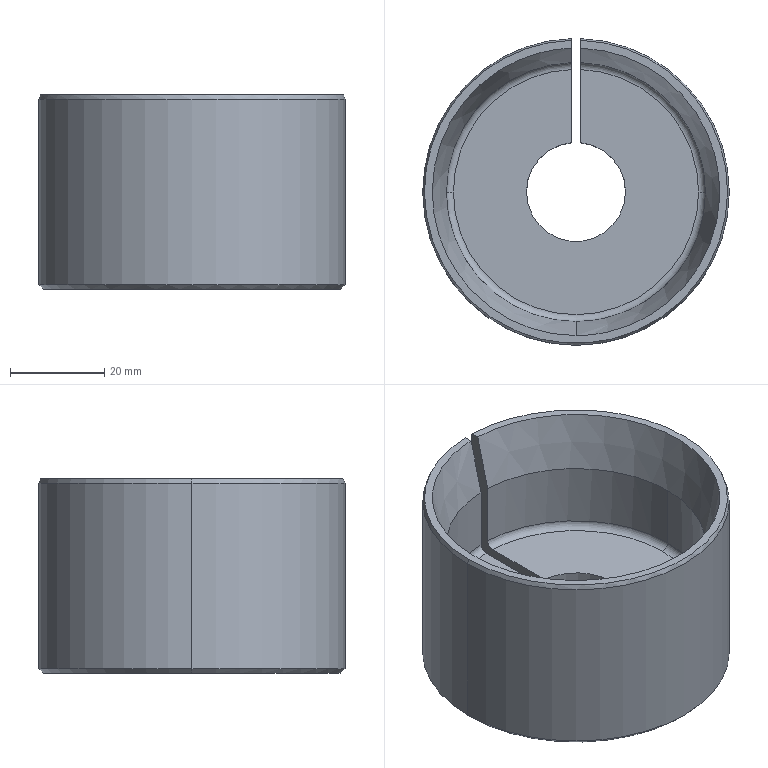Part | SolidWorks | features Chamfer 2, ICE 2, 3DProfileFeature 1, Extrusion 1, Fillet 1, HoleWzd 1, RevCut 1 | 1 solid | 25 faces | box 65 x 64.985 x 41.25 mm | volume 63691 mm3 | cylinder 9 | cone 8 | plane 5 | torus 3 | commonest cylinder face diameters 21 x3 55 x3 65 x3
STEP:
#1=CARTESIAN_POINT('',(-26.,0.,14.25));
#2=VERTEX_POINT('',#1);
#3=CARTESIAN_POINT('',(26.,0.,14.25));
#4=VERTEX_POINT('',#3);
#5=CARTESIAN_POINT('',(0.,0.,14.25));
#6=DIRECTION('',(0.,0.,1.));
#7=DIRECTION('',(1.,0.,0.));
#8=AXIS2_PLACEMENT_3D('',#5,#6,#7);
#9=CIRCLE('',#8,26.);
#10=EDGE_CURVE('',#2,#4,#9,.T.);
#11=ORIENTED_EDGE('',*,*,#10,.F.);
#12=CARTESIAN_POINT('',(-27.5,0.,15.75));
#13=VERTEX_POINT('',#12);
#14=CARTESIAN_POINT('',(-26.,0.,15.75));
#15=DIRECTION('',(0.,1.,0.));
#16=DIRECTION('',(-1.,0.,0.));
#17=AXIS2_PLACEMENT_3D('',#14,#15,#16);
#18=CIRCLE('',#17,1.5);
#19=EDGE_CURVE('',#2,#13,#18,.T.);
#20=ORIENTED_EDGE('',*,*,#19,.T.);
#21=CARTESIAN_POINT('',(27.5,0.,15.75));
#22=VERTEX_POINT('',#21);
#23=CARTESIAN_POINT('',(0.,0.,15.75));
#24=DIRECTION('',(0.,0.,-1.));
#25=DIRECTION('',(1.,0.,0.));
#26=AXIS2_PLACEMENT_3D('',#23,#24,#25);
#27=CIRCLE('',#26,27.5);
#28=EDGE_CURVE('',#22,#13,#27,.T.);
#29=ORIENTED_EDGE('',*,*,#28,.F.);
#30=CARTESIAN_POINT('',(26.,0.,15.75));
#31=DIRECTION('',(0.,-1.,0.));
#32=DIRECTION('',(0.,0.,-1.));
#33=AXIS2_PLACEMENT_3D('',#30,#31,#32);
#34=CIRCLE('',#33,1.5);
#35=EDGE_CURVE('',#4,#22,#34,.T.);
#36=ORIENTED_EDGE('',*,*,#35,.F.);
#37=EDGE_LOOP('',(#11,#20,#29,#36));
#38=FACE_OUTER_BOUND('',#37,.T.);
#39=CARTESIAN_POINT('',(0.,0.,15.75));
#40=DIRECTION('',(0.,0.,1.));
#41=DIRECTION('',(1.,0.,0.));
#42=AXIS2_PLACEMENT_3D('',#39,#40,#41);
#43=TOROIDAL_SURFACE('',#42,26.,1.5);
#44=ADVANCED_FACE('',(#38),#43,.F.);
#45=CARTESIAN_POINT('',(1.,25.981,14.25));
#46=VERTEX_POINT('',#45);
#47=CARTESIAN_POINT('',(0.,0.,14.25));
#48=DIRECTION('',(0.,0.,1.));
#49=DIRECTION('',(1.,0.,0.));
#50=AXIS2_PLACEMENT_3D('',#47,#48,#49);
#51=CIRCLE('',#50,26.);
#52=EDGE_CURVE('',#4,#46,#51,.T.);
#53=ORIENTED_EDGE('',*,*,#52,.F.);
#54=ORIENTED_EDGE('',*,*,#35,.T.);
#55=CARTESIAN_POINT('',(1.,27.482,15.75));
#56=VERTEX_POINT('',#55);
#57=CARTESIAN_POINT('',(0.,0.,15.75));
#58=DIRECTION('',(0.,0.,-1.));
#59=DIRECTION('',(1.,0.,0.));
#60=AXIS2_PLACEMENT_3D('',#57,#58,#59);
#61=CIRCLE('',#60,27.5);
#62=EDGE_CURVE('',#56,#22,#61,.T.);
#63=ORIENTED_EDGE('',*,*,#62,.F.);
#64=CARTESIAN_POINT('',(1.,25.981,14.25));
#65=CARTESIAN_POINT('',(1.,26.08,14.25));
#66=CARTESIAN_POINT('',(1.,26.177,14.26));
#67=CARTESIAN_POINT('',(1.,26.369,14.298));
#68=CARTESIAN_POINT('',(1.,26.464,14.327));
#69=CARTESIAN_POINT('',(1.,26.646,14.402));
#70=CARTESIAN_POINT('',(1.,26.732,14.448));
#71=CARTESIAN_POINT('',(1.,26.895,14.556));
#72=CARTESIAN_POINT('',(1.,26.972,14.62));
#73=CARTESIAN_POINT('',(1.,27.18,14.827));
#74=CARTESIAN_POINT('',(1.,27.292,14.994));
#75=CARTESIAN_POINT('',(1.,27.442,15.355));
#76=CARTESIAN_POINT('',(1.,27.482,15.552));
#77=CARTESIAN_POINT('',(1.,27.482,15.75));
#78=B_SPLINE_CURVE_WITH_KNOTS('',3,(#64,#65,#66,#67,#68,#69,#70,#71,#72,#73,#74,#75,#76,#77),.UNSPECIFIED.,.F.,.F.,(4,2,2,2,2,2,4),(0.,0.000293,0.000586,0.000879,0.001172,0.001758,0.002344),.UNSPECIFIED.);
#79=EDGE_CURVE('',#46,#56,#78,.T.);
#80=ORIENTED_EDGE('',*,*,#79,.F.);
#81=EDGE_LOOP('',(#53,#54,#63,#80));
#82=FACE_OUTER_BOUND('',#81,.T.);
#83=CARTESIAN_POINT('',(0.,0.,15.75));
#84=DIRECTION('',(0.,0.,1.));
#85=DIRECTION('',(1.,0.,0.));
#86=AXIS2_PLACEMENT_3D('',#83,#84,#85);
#87=TOROIDAL_SURFACE('',#86,26.,1.5);
#88=ADVANCED_FACE('',(#82),#87,.F.);
#89=CARTESIAN_POINT('',(32.136,0.,41.25));
#90=VERTEX_POINT('',#89);
#91=CARTESIAN_POINT('',(1.,32.12,41.25));
#92=VERTEX_POINT('',#91);
#93=CARTESIAN_POINT('',(0.,0.,41.25));
#94=DIRECTION('',(0.,0.,1.));
#95=DIRECTION('',(1.,0.,0.));
#96=AXIS2_PLACEMENT_3D('',#93,#94,#95);
#97=CIRCLE('',#96,32.136);
#98=EDGE_CURVE('',#90,#92,#97,.T.);
#99=ORIENTED_EDGE('',*,*,#98,.F.);
#100=CARTESIAN_POINT('',(32.5,0.,40.25));
#101=VERTEX_POINT('',#100);
#102=CARTESIAN_POINT('',(32.136,0.,41.25));
#103=DIRECTION('',(0.342,0.,-0.9397));
#104=VECTOR('',#103,1000.);
#105=LINE('',#102,#104);
#106=EDGE_CURVE('',#90,#101,#105,.T.);
#107=ORIENTED_EDGE('',*,*,#106,.T.);
#108=CARTESIAN_POINT('',(1.,32.485,40.25));
#109=VERTEX_POINT('',#108);
#110=CARTESIAN_POINT('',(0.,0.,40.25));
#111=DIRECTION('',(0.,0.,-1.));
#112=DIRECTION('',(1.,0.,0.));
#113=AXIS2_PLACEMENT_3D('',#110,#111,#112);
#114=CIRCLE('',#113,32.5);
#115=EDGE_CURVE('',#109,#101,#114,.T.);
#116=ORIENTED_EDGE('',*,*,#115,.F.);
#117=CARTESIAN_POINT('',(1.,32.12,41.25));
#118=CARTESIAN_POINT('',(1.,32.242,40.917));
#119=CARTESIAN_POINT('',(1.,32.363,40.583));
#120=CARTESIAN_POINT('',(1.,32.485,40.25));
#121=B_SPLINE_CURVE_WITH_KNOTS('',3,(#117,#118,#119,#120),.UNSPECIFIED.,.F.,.F.,(4,4),(0.,0.001064),.UNSPECIFIED.);
#122=EDGE_CURVE('',#92,#109,#121,.T.);
#123=ORIENTED_EDGE('',*,*,#122,.F.);
#124=EDGE_LOOP('',(#99,#107,#116,#123));
#125=FACE_OUTER_BOUND('',#124,.T.);
#126=CARTESIAN_POINT('',(0.,0.,41.25));
#127=DIRECTION('',(0.,0.,-1.));
#128=DIRECTION('',(-1.,0.,0.));
#129=AXIS2_PLACEMENT_3D('',#126,#127,#128);
#130=CONICAL_SURFACE('',#129,32.136,0.3491);
#131=ADVANCED_FACE('',(#125),#130,.T.);
#132=ORIENTED_EDGE('',*,*,#106,.F.);
#133=CARTESIAN_POINT('',(-32.136,0.,41.25));
#134=VERTEX_POINT('',#133);
#135=CARTESIAN_POINT('',(0.,0.,41.25));
#136=DIRECTION('',(0.,0.,1.));
#137=DIRECTION('',(1.,0.,0.));
#138=AXIS2_PLACEMENT_3D('',#135,#136,#137);
#139=CIRCLE('',#138,32.136);
#140=EDGE_CURVE('',#134,#90,#139,.T.);
#141=ORIENTED_EDGE('',*,*,#140,.F.);
#142=CARTESIAN_POINT('',(-32.5,0.,40.25));
#143=VERTEX_POINT('',#142);
#144=CARTESIAN_POINT('',(-32.136,0.,41.25));
#145=DIRECTION('',(-0.342,0.,-0.9397));
#146=VECTOR('',#145,1000.);
#147=LINE('',#144,#146);
#148=EDGE_CURVE('',#134,#143,#147,.T.);
#149=ORIENTED_EDGE('',*,*,#148,.T.);
#150=CARTESIAN_POINT('',(0.,0.,40.25));
#151=DIRECTION('',(0.,0.,-1.));
#152=DIRECTION('',(1.,0.,0.));
#153=AXIS2_PLACEMENT_3D('',#150,#151,#152);
#154=CIRCLE('',#153,32.5);
#155=EDGE_CURVE('',#101,#143,#154,.T.);
#156=ORIENTED_EDGE('',*,*,#155,.F.);
#157=EDGE_LOOP('',(#132,#141,#149,#156));
#158=FACE_OUTER_BOUND('',#157,.T.);
#159=CARTESIAN_POINT('',(0.,0.,41.25));
#160=DIRECTION('',(0.,0.,-1.));
#161=DIRECTION('',(-1.,0.,0.));
#162=AXIS2_PLACEMENT_3D('',#159,#160,#161);
#163=CONICAL_SURFACE('',#162,32.136,0.3491);
#164=ADVANCED_FACE('',(#158),#163,.T.);
#165=CARTESIAN_POINT('',(-31.5,0.,0.));
#166=VERTEX_POINT('',#165);
#167=CARTESIAN_POINT('',(-1.,31.484,0.));
#168=VERTEX_POINT('',#167);
#169=CARTESIAN_POINT('',(0.,0.,0.));
#170=DIRECTION('',(0.,0.,-1.));
#171=DIRECTION('',(1.,0.,0.));
#172=AXIS2_PLACEMENT_3D('',#169,#170,#171);
#173=CIRCLE('',#172,31.5);
#174=EDGE_CURVE('',#166,#168,#173,.T.);
#175=ORIENTED_EDGE('',*,*,#174,.F.);
#176=CARTESIAN_POINT('',(-32.5,0.,1.));
#177=VERTEX_POINT('',#176);
#178=CARTESIAN_POINT('',(-32.5,0.,1.));
#179=DIRECTION('',(-0.7071,0.,0.7071));
#180=VECTOR('',#179,1000.);
#181=LINE('',#178,#180);
#182=EDGE_CURVE('',#166,#177,#181,.T.);
#183=ORIENTED_EDGE('',*,*,#182,.T.);
#184=CARTESIAN_POINT('',(-1.,32.485,1.));
#185=VERTEX_POINT('',#184);
#186=CARTESIAN_POINT('',(0.,0.,1.));
#187=DIRECTION('',(0.,0.,1.));
#188=DIRECTION('',(1.,0.,0.));
#189=AXIS2_PLACEMENT_3D('',#186,#187,#188);
#190=CIRCLE('',#189,32.5);
#191=EDGE_CURVE('',#185,#177,#190,.T.);
#192=ORIENTED_EDGE('',*,*,#191,.F.);
#193=CARTESIAN_POINT('',(-1.,31.484,0.));
#194=CARTESIAN_POINT('',(-1.,31.818,0.3333));
#195=CARTESIAN_POINT('',(-1.,32.151,0.6667));
#196=CARTESIAN_POINT('',(-1.,32.485,1.));
#197=B_SPLINE_CURVE_WITH_KNOTS('',3,(#193,#194,#195,#196),.UNSPECIFIED.,.F.,.F.,(4,4),(0.,0.001415),.UNSPECIFIED.);
#198=EDGE_CURVE('',#168,#185,#197,.T.);
#199=ORIENTED_EDGE('',*,*,#198,.F.);
#200=EDGE_LOOP('',(#175,#183,#192,#199));
#201=FACE_OUTER_BOUND('',#200,.T.);
#202=CARTESIAN_POINT('',(0.,0.,1.));
#203=DIRECTION('',(0.,0.,1.));
#204=DIRECTION('',(1.,0.,0.));
#205=AXIS2_PLACEMENT_3D('',#202,#203,#204);
#206=CONICAL_SURFACE('',#205,32.5,0.7854);
#207=ADVANCED_FACE('',(#201),#206,.T.);
#208=ORIENTED_EDGE('',*,*,#182,.F.);
#209=CARTESIAN_POINT('',(31.5,0.,0.));
#210=VERTEX_POINT('',#209);
#211=CARTESIAN_POINT('',(0.,0.,0.));
#212=DIRECTION('',(0.,0.,-1.));
#213=DIRECTION('',(1.,0.,0.));
#214=AXIS2_PLACEMENT_3D('',#211,#212,#213);
#215=CIRCLE('',#214,31.5);
#216=EDGE_CURVE('',#210,#166,#215,.T.);
#217=ORIENTED_EDGE('',*,*,#216,.F.);
#218=CARTESIAN_POINT('',(32.5,0.,1.));
#219=VERTEX_POINT('',#218);
#220=CARTESIAN_POINT('',(32.5,0.,1.));
#221=DIRECTION('',(0.7071,0.,0.7071));
#222=VECTOR('',#221,1000.);
#223=LINE('',#220,#222);
#224=EDGE_CURVE('',#210,#219,#223,.T.);
#225=ORIENTED_EDGE('',*,*,#224,.T.);
#226=CARTESIAN_POINT('',(0.,0.,1.));
#227=DIRECTION('',(0.,0.,1.));
#228=DIRECTION('',(1.,0.,0.));
#229=AXIS2_PLACEMENT_3D('',#226,#227,#228);
#230=CIRCLE('',#229,32.5);
#231=EDGE_CURVE('',#177,#219,#230,.T.);
#232=ORIENTED_EDGE('',*,*,#231,.F.);
#233=EDGE_LOOP('',(#208,#217,#225,#232));
#234=FACE_OUTER_BOUND('',#233,.T.);
#235=CARTESIAN_POINT('',(0.,0.,1.));
#236=DIRECTION('',(0.,0.,1.));
#237=DIRECTION('',(1.,0.,0.));
#238=AXIS2_PLACEMENT_3D('',#235,#236,#237);
#239=CONICAL_SURFACE('',#238,32.5,0.7854);
#240=ADVANCED_FACE('',(#234),#239,.T.);
#241=CARTESIAN_POINT('',(27.5,0.,29.296));
#242=VERTEX_POINT('',#241);
#243=CARTESIAN_POINT('',(0.,-27.5,29.269));
#244=VERTEX_POINT('',#243);
#245=CARTESIAN_POINT('',(27.5,0.,29.296));
#246=CARTESIAN_POINT('',(27.5,-0.8956,29.295));
#247=CARTESIAN_POINT('',(27.456,-1.792,29.294));
#248=CARTESIAN_POINT('',(27.28,-3.586,29.292));
#249=CARTESIAN_POINT('',(27.146,-4.488,29.291));
#250=CARTESIAN_POINT('',(26.617,-7.143,29.289));
#251=CARTESIAN_POINT('',(26.096,-8.857,29.287));
#252=CARTESIAN_POINT('',(25.067,-11.346,29.285));
#253=CARTESIAN_POINT('',(24.681,-12.162,29.284));
#254=CARTESIAN_POINT('',(23.825,-13.764,29.282));
#255=CARTESIAN_POINT('',(23.361,-14.537,29.282));
#256=CARTESIAN_POINT('',(21.865,-16.775,29.279));
#257=CARTESIAN_POINT('',(20.729,-18.161,29.278));
#258=CARTESIAN_POINT('',(18.815,-20.077,29.276));
#259=CARTESIAN_POINT('',(18.139,-20.689,29.276));
#260=CARTESIAN_POINT('',(16.746,-21.832,29.274));
#261=CARTESIAN_POINT('',(16.025,-22.366,29.274));
#262=CARTESIAN_POINT('',(14.536,-23.362,29.273));
#263=CARTESIAN_POINT('',(13.768,-23.823,29.273));
#264=CARTESIAN_POINT('',(12.579,-24.458,29.272));
#265=CARTESIAN_POINT('',(12.177,-24.661,29.272));
#266=CARTESIAN_POINT('',(11.36,-25.048,29.271));
#267=CARTESIAN_POINT('',(10.945,-25.232,29.271));
#268=CARTESIAN_POINT('',(8.852,-26.099,29.27));
#269=CARTESIAN_POINT('',(7.135,-26.619,29.27));
#270=CARTESIAN_POINT('',(4.498,-27.144,29.269));
#271=CARTESIAN_POINT('',(3.609,-27.277,29.269));
#272=CARTESIAN_POINT('',(2.259,-27.411,29.269));
#273=CARTESIAN_POINT('',(1.805,-27.444,29.269));
#274=CARTESIAN_POINT('',(0.901,-27.489,29.269));
#275=CARTESIAN_POINT('',(0.45,-27.5,29.269));
#276=CARTESIAN_POINT('',(0.,-27.5,29.269));
#277=B_SPLINE_CURVE_WITH_KNOTS('',3,(#245,#246,#247,#248,#249,#250,#251,#252,#253,#254,#255,#256,#257,#258,#259,#260,#261,#262,#263,#264,#265,#266,#267,#268,#269,#270,#271,#272,#273,#274,#275,#276),.UNSPECIFIED.,.F.,.F.,(4,2,2,2,2,2,2,2,2,2,2,2,2,2,2,4),(0.042,0.04469,0.04738,0.05275,0.05544,0.05812,0.0635,0.06618,0.06887,0.07155,0.0729,0.07424,0.07961,0.0823,0.08364,0.08499),.UNSPECIFIED.);
#278=EDGE_CURVE('',#242,#244,#277,.T.);
#279=ORIENTED_EDGE('',*,*,#278,.T.);
#280=CARTESIAN_POINT('',(0.,-30.492,41.25));
#281=VERTEX_POINT('',#280);
#282=CARTESIAN_POINT('',(0.,-27.493,29.24));
#283=DIRECTION('',(0.,-0.2423,0.9702));
#284=VECTOR('',#283,1000.);
#285=LINE('',#282,#284);
#286=EDGE_CURVE('',#244,#281,#285,.T.);
#287=ORIENTED_EDGE('',*,*,#286,.T.);
#288=CARTESIAN_POINT('',(1.,30.457,41.25));
#289=VERTEX_POINT('',#288);
#290=CARTESIAN_POINT('',(1.,30.457,41.25));
#291=CARTESIAN_POINT('',(59.989,28.521,41.25));
#292=CARTESIAN_POINT('',(59.021,-30.492,41.25));
#293=CARTESIAN_POINT('',(0.,-30.492,41.25));
#294=(BOUNDED_CURVE()B_SPLINE_CURVE(3,(#290,#291,#292,#293),.UNSPECIFIED.,.F.,.T.)B_SPLINE_CURVE_WITH_KNOTS((4,4),(3.174,6.283),.UNSPECIFIED.)CURVE()GEOMETRIC_REPRESENTATION_ITEM()RATIONAL_B_SPLINE_CURVE((1.,0.3443,0.3443,1.))REPRESENTATION_ITEM(''));
#295=EDGE_CURVE('',#289,#281,#294,.T.);
#296=ORIENTED_EDGE('',*,*,#295,.F.);
#297=CARTESIAN_POINT('',(1.,27.482,29.323));
#298=VERTEX_POINT('',#297);
#299=CARTESIAN_POINT('',(1.,30.457,41.25));
#300=CARTESIAN_POINT('',(1.,29.466,37.274));
#301=CARTESIAN_POINT('',(1.,28.474,33.299));
#302=CARTESIAN_POINT('',(1.,27.482,29.323));
#303=B_SPLINE_CURVE_WITH_KNOTS('',3,(#299,#300,#301,#302),.UNSPECIFIED.,.F.,.F.,(4,4),(0.02473,0.03702),.UNSPECIFIED.);
#304=EDGE_CURVE('',#289,#298,#303,.T.);
#305=ORIENTED_EDGE('',*,*,#304,.T.);
#306=CARTESIAN_POINT('',(1.,27.482,29.323));
#307=CARTESIAN_POINT('',(2.774,27.417,29.323));
#308=CARTESIAN_POINT('',(4.513,27.184,29.323));
#309=CARTESIAN_POINT('',(7.07,26.59,29.322));
#310=CARTESIAN_POINT('',(7.914,26.351,29.322));
#311=CARTESIAN_POINT('',(9.585,25.79,29.321));
#312=CARTESIAN_POINT('',(10.415,25.467,29.321));
#313=CARTESIAN_POINT('',(12.83,24.388,29.32));
#314=CARTESIAN_POINT('',(14.352,23.523,29.319));
#315=CARTESIAN_POINT('',(16.507,22.013,29.318));
#316=CARTESIAN_POINT('',(17.203,21.473,29.317));
#317=CARTESIAN_POINT('',(18.551,20.32,29.316));
#318=CARTESIAN_POINT('',(19.193,19.714,29.315));
#319=CARTESIAN_POINT('',(21.02,17.818,29.313));
#320=CARTESIAN_POINT('',(22.109,16.448,29.312));
#321=CARTESIAN_POINT('',(23.548,14.232,29.31));
#322=CARTESIAN_POINT('',(23.996,13.462,29.309));
#323=CARTESIAN_POINT('',(24.809,11.897,29.308));
#324=CARTESIAN_POINT('',(25.176,11.099,29.307));
#325=CARTESIAN_POINT('',(26.158,8.664,29.304));
#326=CARTESIAN_POINT('',(26.658,6.983,29.303));
#327=CARTESIAN_POINT('',(27.165,4.372,29.3));
#328=CARTESIAN_POINT('',(27.291,3.497,29.299));
#329=CARTESIAN_POINT('',(27.458,1.75,29.298));
#330=CARTESIAN_POINT('',(27.5,0.8751,29.297));
#331=CARTESIAN_POINT('',(27.5,0.,29.296));
#332=B_SPLINE_CURVE_WITH_KNOTS('',3,(#306,#307,#308,#309,#310,#311,#312,#313,#314,#315,#316,#317,#318,#319,#320,#321,#322,#323,#324,#325,#326,#327,#328,#329,#330,#331),.UNSPECIFIED.,.F.,.F.,(4,2,2,2,2,2,2,2,2,2,2,2,4),(0.000005437,0.005255,0.00788,0.01051,0.01576,0.01838,0.021,0.02625,0.02888,0.0315,0.03675,0.03938,0.042),.UNSPECIFIED.);
#333=EDGE_CURVE('',#298,#242,#332,.T.);
#334=ORIENTED_EDGE('',*,*,#333,.T.);
#335=EDGE_LOOP('',(#279,#287,#296,#305,#334));
#336=FACE_OUTER_BOUND('',#335,.T.);
#337=CARTESIAN_POINT('',(0.,-0.005455,29.245));
#338=DIRECTION('',(0.,-0.0001865,1.));
#339=DIRECTION('',(0.,-1.,-0.0001865));
#340=AXIS2_PLACEMENT_3D('',#337,#338,#339);
#341=CONICAL_SURFACE('',#340,27.487,0.2445);
#342=ADVANCED_FACE('',(#336),#341,.F.);
#343=CARTESIAN_POINT('',(-10.5,0.,14.25));
#344=VERTEX_POINT('',#343);
#345=CARTESIAN_POINT('',(10.5,0.,14.25));
#346=VERTEX_POINT('',#345);
#347=CARTESIAN_POINT('',(0.,0.,14.25));
#348=DIRECTION('',(0.,0.,1.));
#349=DIRECTION('',(1.,0.,0.));
#350=AXIS2_PLACEMENT_3D('',#347,#348,#349);
#351=CIRCLE('',#350,10.5);
#352=EDGE_CURVE('',#344,#346,#351,.T.);
#353=ORIENTED_EDGE('',*,*,#352,.T.);
#354=CARTESIAN_POINT('',(10.5,0.,0.));
#355=VERTEX_POINT('',#354);
#356=CARTESIAN_POINT('',(10.5,0.,0.));
#357=DIRECTION('',(0.,0.,-1.));
#358=VECTOR('',#357,1000.);
#359=LINE('',#356,#358);
#360=EDGE_CURVE('',#346,#355,#359,.T.);
#361=ORIENTED_EDGE('',*,*,#360,.T.);
#362=CARTESIAN_POINT('',(-10.5,0.,0.));
#363=VERTEX_POINT('',#362);
#364=CARTESIAN_POINT('',(0.,0.,0.));
#365=DIRECTION('',(0.,0.,-1.));
#366=DIRECTION('',(-1.,0.,0.));
#367=AXIS2_PLACEMENT_3D('',#364,#365,#366);
#368=CIRCLE('',#367,10.5);
#369=EDGE_CURVE('',#355,#363,#368,.T.);
#370=ORIENTED_EDGE('',*,*,#369,.T.);
#371=CARTESIAN_POINT('',(-10.5,0.,0.));
#372=DIRECTION('',(0.,0.,-1.));
#373=VECTOR('',#372,1000.);
#374=LINE('',#371,#373);
#375=EDGE_CURVE('',#344,#363,#374,.T.);
#376=ORIENTED_EDGE('',*,*,#375,.F.);
#377=EDGE_LOOP('',(#353,#361,#370,#376));
#378=FACE_OUTER_BOUND('',#377,.T.);
#379=CARTESIAN_POINT('',(0.,0.,0.));
#380=DIRECTION('',(0.,0.,-1.));
#381=DIRECTION('',(-1.,0.,0.));
#382=AXIS2_PLACEMENT_3D('',#379,#380,#381);
#383=CYLINDRICAL_SURFACE('',#382,10.5);
#384=ADVANCED_FACE('',(#378),#383,.F.);
#385=CARTESIAN_POINT('',(-1.,10.452,14.25));
#386=VERTEX_POINT('',#385);
#387=CARTESIAN_POINT('',(0.,0.,14.25));
#388=DIRECTION('',(0.,0.,1.));
#389=DIRECTION('',(1.,0.,0.));
#390=AXIS2_PLACEMENT_3D('',#387,#388,#389);
#391=CIRCLE('',#390,10.5);
#392=EDGE_CURVE('',#386,#344,#391,.T.);
#393=ORIENTED_EDGE('',*,*,#392,.T.);
#394=ORIENTED_EDGE('',*,*,#375,.T.);
#395=CARTESIAN_POINT('',(-1.,10.452,0.));
#396=VERTEX_POINT('',#395);
#397=CARTESIAN_POINT('',(0.,0.,0.));
#398=DIRECTION('',(0.,0.,-1.));
#399=DIRECTION('',(-1.,0.,0.));
#400=AXIS2_PLACEMENT_3D('',#397,#398,#399);
#401=CIRCLE('',#400,10.5);
#402=EDGE_CURVE('',#363,#396,#401,.T.);
#403=ORIENTED_EDGE('',*,*,#402,.T.);
#404=CARTESIAN_POINT('',(-1.,10.452,0.));
#405=DIRECTION('',(0.,0.,1.));
#406=VECTOR('',#405,1000.);
#407=LINE('',#404,#406);
#408=EDGE_CURVE('',#396,#386,#407,.T.);
#409=ORIENTED_EDGE('',*,*,#408,.T.);
#410=EDGE_LOOP('',(#393,#394,#403,#409));
#411=FACE_OUTER_BOUND('',#410,.T.);
#412=CARTESIAN_POINT('',(0.,0.,0.));
#413=DIRECTION('',(0.,0.,-1.));
#414=DIRECTION('',(-1.,0.,0.));
#415=AXIS2_PLACEMENT_3D('',#412,#413,#414);
#416=CYLINDRICAL_SURFACE('',#415,10.5);
#417=ADVANCED_FACE('',(#411),#416,.F.);
#418=ORIENTED_EDGE('',*,*,#115,.T.);
#419=CARTESIAN_POINT('',(32.5,0.,41.25));
#420=DIRECTION('',(0.,0.,-1.));
#421=VECTOR('',#420,1000.);
#422=LINE('',#419,#421);
#423=EDGE_CURVE('',#101,#219,#422,.T.);
#424=ORIENTED_EDGE('',*,*,#423,.T.);
#425=CARTESIAN_POINT('',(1.,32.485,1.));
#426=VERTEX_POINT('',#425);
#427=CARTESIAN_POINT('',(0.,0.,1.));
#428=DIRECTION('',(0.,0.,1.));
#429=DIRECTION('',(1.,0.,0.));
#430=AXIS2_PLACEMENT_3D('',#427,#428,#429);
#431=CIRCLE('',#430,32.5);
#432=EDGE_CURVE('',#219,#426,#431,.T.);
#433=ORIENTED_EDGE('',*,*,#432,.T.);
#434=CARTESIAN_POINT('',(1.,32.485,41.25));
#435=DIRECTION('',(0.,0.,1.));
#436=VECTOR('',#435,1000.);
#437=LINE('',#434,#436);
#438=EDGE_CURVE('',#426,#109,#437,.T.);
#439=ORIENTED_EDGE('',*,*,#438,.T.);
#440=EDGE_LOOP('',(#418,#424,#433,#439));
#441=FACE_OUTER_BOUND('',#440,.T.);
#442=CARTESIAN_POINT('',(0.,0.,41.25));
#443=DIRECTION('',(0.,0.,-1.));
#444=DIRECTION('',(-1.,0.,0.));
#445=AXIS2_PLACEMENT_3D('',#442,#443,#444);
#446=CYLINDRICAL_SURFACE('',#445,32.5);
#447=ADVANCED_FACE('',(#441),#446,.T.);
#448=ORIENTED_EDGE('',*,*,#423,.F.);
#449=ORIENTED_EDGE('',*,*,#155,.T.);
#450=CARTESIAN_POINT('',(-32.5,0.,41.25));
#451=DIRECTION('',(0.,0.,-1.));
#452=VECTOR('',#451,1000.);
#453=LINE('',#450,#452);
#454=EDGE_CURVE('',#143,#177,#453,.T.);
#455=ORIENTED_EDGE('',*,*,#454,.T.);
#456=ORIENTED_EDGE('',*,*,#231,.T.);
#457=EDGE_LOOP('',(#448,#449,#455,#456));
#458=FACE_OUTER_BOUND('',#457,.T.);
#459=CARTESIAN_POINT('',(0.,0.,41.25));
#460=DIRECTION('',(0.,0.,-1.));
#461=DIRECTION('',(-1.,0.,0.));
#462=AXIS2_PLACEMENT_3D('',#459,#460,#461);
#463=CYLINDRICAL_SURFACE('',#462,32.5);
#464=ADVANCED_FACE('',(#458),#463,.T.);
#465=ORIENTED_EDGE('',*,*,#28,.T.);
#466=CARTESIAN_POINT('',(-27.5,0.,29.296));
#467=VERTEX_POINT('',#466);
#468=CARTESIAN_POINT('',(-27.5,0.,14.25));
#469=DIRECTION('',(0.,0.,1.));
#470=VECTOR('',#469,1000.);
#471=LINE('',#468,#470);
#472=EDGE_CURVE('',#13,#467,#471,.T.);
#473=ORIENTED_EDGE('',*,*,#472,.T.);
#474=CARTESIAN_POINT('',(0.,-27.5,29.269));
#475=CARTESIAN_POINT('',(-1.801,-27.5,29.269));
#476=CARTESIAN_POINT('',(-3.584,-27.325,29.269));
#477=CARTESIAN_POINT('',(-5.792,-26.887,29.269));
#478=CARTESIAN_POINT('',(-6.232,-26.788,29.27));
#479=CARTESIAN_POINT('',(-7.111,-26.569,29.27));
#480=CARTESIAN_POINT('',(-7.55,-26.447,29.27));
#481=CARTESIAN_POINT('',(-8.849,-26.053,29.27));
#482=CARTESIAN_POINT('',(-9.696,-25.75,29.271));
#483=CARTESIAN_POINT('',(-12.182,-24.72,29.272));
#484=CARTESIAN_POINT('',(-13.765,-23.876,29.272));
#485=CARTESIAN_POINT('',(-15.65,-22.617,29.274));
#486=CARTESIAN_POINT('',(-16.022,-22.355,29.274));
#487=CARTESIAN_POINT('',(-16.748,-21.816,29.274));
#488=CARTESIAN_POINT('',(-17.104,-21.539,29.275));
#489=CARTESIAN_POINT('',(-18.146,-20.683,29.276));
#490=CARTESIAN_POINT('',(-18.81,-20.08,29.276));
#491=CARTESIAN_POINT('',(-20.078,-18.813,29.277));
#492=CARTESIAN_POINT('',(-20.681,-18.148,29.278));
#493=CARTESIAN_POINT('',(-21.825,-16.755,29.279));
#494=CARTESIAN_POINT('',(-22.368,-16.023,29.28));
#495=CARTESIAN_POINT('',(-23.874,-13.768,29.282));
#496=CARTESIAN_POINT('',(-24.718,-12.186,29.284));
#497=CARTESIAN_POINT('',(-25.749,-9.698,29.286));
#498=CARTESIAN_POINT('',(-26.053,-8.849,29.287));
#499=CARTESIAN_POINT('',(-26.58,-7.11,29.289));
#500=CARTESIAN_POINT('',(-26.799,-6.233,29.29));
#501=CARTESIAN_POINT('',(-27.324,-3.589,29.292));
#502=CARTESIAN_POINT('',(-27.5,-1.805,29.294));
#503=CARTESIAN_POINT('',(-27.5,0.,29.296));
#504=B_SPLINE_CURVE_WITH_KNOTS('',3,(#474,#475,#476,#477,#478,#479,#480,#481,#482,#483,#484,#485,#486,#487,#488,#489,#490,#491,#492,#493,#494,#495,#496,#497,#498,#499,#500,#501,#502,#503),.UNSPECIFIED.,.F.,.F.,(4,2,2,2,2,2,2,2,2,2,2,2,2,2,4),(0.08499,0.09036,0.09171,0.09305,0.09574,0.1011,0.1025,0.1038,0.1065,0.1092,0.1119,0.1172,0.1199,0.1226,0.128),.UNSPECIFIED.);
#505=EDGE_CURVE('',#244,#467,#504,.T.);
#506=ORIENTED_EDGE('',*,*,#505,.F.);
#507=ORIENTED_EDGE('',*,*,#278,.F.);
#508=CARTESIAN_POINT('',(27.5,0.,14.25));
#509=DIRECTION('',(0.,0.,1.));
#510=VECTOR('',#509,1000.);
#511=LINE('',#508,#510);
#512=EDGE_CURVE('',#22,#242,#511,.T.);
#513=ORIENTED_EDGE('',*,*,#512,.F.);
#514=EDGE_LOOP('',(#465,#473,#506,#507,#513));
#515=FACE_OUTER_BOUND('',#514,.T.);
#516=CARTESIAN_POINT('',(0.,0.,14.25));
#517=DIRECTION('',(0.,0.,1.));
#518=DIRECTION('',(1.,0.,0.));
#519=AXIS2_PLACEMENT_3D('',#516,#517,#518);
#520=CYLINDRICAL_SURFACE('',#519,27.5);
#521=ADVANCED_FACE('',(#515),#520,.F.);
#522=ORIENTED_EDGE('',*,*,#62,.T.);
#523=ORIENTED_EDGE('',*,*,#512,.T.);
#524=ORIENTED_EDGE('',*,*,#333,.F.);
#525=CARTESIAN_POINT('',(1.,27.482,14.25));
#526=DIRECTION('',(0.,0.,-1.));
#527=VECTOR('',#526,1000.);
#528=LINE('',#525,#527);
#529=EDGE_CURVE('',#298,#56,#528,.T.);
#530=ORIENTED_EDGE('',*,*,#529,.T.);
#531=EDGE_LOOP('',(#522,#523,#524,#530));
#532=FACE_OUTER_BOUND('',#531,.T.);
#533=CARTESIAN_POINT('',(0.,0.,14.25));
#534=DIRECTION('',(0.,0.,1.));
#535=DIRECTION('',(1.,0.,0.));
#536=AXIS2_PLACEMENT_3D('',#533,#534,#535);
#537=CYLINDRICAL_SURFACE('',#536,27.5);
#538=ADVANCED_FACE('',(#532),#537,.F.);
#539=ORIENTED_EDGE('',*,*,#472,.F.);
#540=CARTESIAN_POINT('',(-1.,27.482,15.75));
#541=VERTEX_POINT('',#540);
#542=CARTESIAN_POINT('',(0.,0.,15.75));
#543=DIRECTION('',(0.,0.,-1.));
#544=DIRECTION('',(1.,0.,0.));
#545=AXIS2_PLACEMENT_3D('',#542,#543,#544);
#546=CIRCLE('',#545,27.5);
#547=EDGE_CURVE('',#13,#541,#546,.T.);
#548=ORIENTED_EDGE('',*,*,#547,.T.);
#549=CARTESIAN_POINT('',(-1.,27.482,29.323));
#550=VERTEX_POINT('',#549);
#551=CARTESIAN_POINT('',(-1.,27.482,14.25));
#552=DIRECTION('',(0.,0.,1.));
#553=VECTOR('',#552,1000.);
#554=LINE('',#551,#553);
#555=EDGE_CURVE('',#541,#550,#554,.T.);
#556=ORIENTED_EDGE('',*,*,#555,.T.);
#557=CARTESIAN_POINT('',(-27.5,0.,29.296));
#558=CARTESIAN_POINT('',(-27.5,0.8807,29.297));
#559=CARTESIAN_POINT('',(-27.457,1.77,29.298));
#560=CARTESIAN_POINT('',(-27.288,3.523,29.299));
#561=CARTESIAN_POINT('',(-27.161,4.39,29.3));
#562=CARTESIAN_POINT('',(-26.661,6.965,29.303));
#563=CARTESIAN_POINT('',(-26.166,8.646,29.304));
#564=CARTESIAN_POINT('',(-24.839,11.935,29.308));
#565=CARTESIAN_POINT('',(-24.028,13.49,29.309));
#566=CARTESIAN_POINT('',(-22.601,15.691,29.311));
#567=CARTESIAN_POINT('',(-22.09,16.403,29.312));
#568=CARTESIAN_POINT('',(-20.996,17.782,29.313));
#569=CARTESIAN_POINT('',(-20.41,18.452,29.314));
#570=CARTESIAN_POINT('',(-18.576,20.354,29.316));
#571=CARTESIAN_POINT('',(-17.247,21.491,29.317));
#572=CARTESIAN_POINT('',(-15.096,23.003,29.319));
#573=CARTESIAN_POINT('',(-14.353,23.474,29.319));
#574=CARTESIAN_POINT('',(-12.812,24.349,29.32));
#575=CARTESIAN_POINT('',(-12.025,24.747,29.32));
#576=CARTESIAN_POINT('',(-9.624,25.821,29.321));
#577=CARTESIAN_POINT('',(-7.967,26.38,29.322));
#578=CARTESIAN_POINT('',(-5.396,26.98,29.322));
#579=CARTESIAN_POINT('',(-4.522,27.14,29.323));
#580=CARTESIAN_POINT('',(-2.768,27.375,29.323));
#581=CARTESIAN_POINT('',(-1.886,27.45,29.323));
#582=CARTESIAN_POINT('',(-1.,27.482,29.323));
#583=B_SPLINE_CURVE_WITH_KNOTS('',3,(#557,#558,#559,#560,#561,#562,#563,#564,#565,#566,#567,#568,#569,#570,#571,#572,#573,#574,#575,#576,#577,#578,#579,#580,#581,#582),.UNSPECIFIED.,.F.,.F.,(4,2,2,2,2,2,2,2,2,2,2,2,4),(0.128,0.1306,0.1332,0.1385,0.1437,0.1464,0.149,0.1542,0.1568,0.1595,0.1647,0.1673,0.17),.UNSPECIFIED.);
#584=EDGE_CURVE('',#467,#550,#583,.T.);
#585=ORIENTED_EDGE('',*,*,#584,.F.);
#586=EDGE_LOOP('',(#539,#548,#556,#585));
#587=FACE_OUTER_BOUND('',#586,.T.);
#588=CARTESIAN_POINT('',(0.,0.,14.25));
#589=DIRECTION('',(0.,0.,1.));
#590=DIRECTION('',(1.,0.,0.));
#591=AXIS2_PLACEMENT_3D('',#588,#589,#590);
#592=CYLINDRICAL_SURFACE('',#591,27.5);
#593=ADVANCED_FACE('',(#587),#592,.F.);
#594=CARTESIAN_POINT('',(1.,37.064,41.25));
#595=DIRECTION('',(0.,-1.,0.));
#596=VECTOR('',#595,1000.);
#597=LINE('',#594,#596);
#598=EDGE_CURVE('',#92,#289,#597,.T.);
#599=ORIENTED_EDGE('',*,*,#598,.F.);
#600=ORIENTED_EDGE('',*,*,#122,.T.);
#601=ORIENTED_EDGE('',*,*,#438,.F.);
#602=CARTESIAN_POINT('',(1.,31.484,0.));
#603=VERTEX_POINT('',#602);
#604=CARTESIAN_POINT('',(1.,32.485,1.));
#605=CARTESIAN_POINT('',(1.,32.151,0.6667));
#606=CARTESIAN_POINT('',(1.,31.818,0.3333));
#607=CARTESIAN_POINT('',(1.,31.484,0.));
#608=B_SPLINE_CURVE_WITH_KNOTS('',3,(#604,#605,#606,#607),.UNSPECIFIED.,.F.,.F.,(4,4),(0.,0.001415),.UNSPECIFIED.);
#609=EDGE_CURVE('',#426,#603,#608,.T.);
#610=ORIENTED_EDGE('',*,*,#609,.T.);
#611=CARTESIAN_POINT('',(1.,10.452,0.));
#612=VERTEX_POINT('',#611);
#613=CARTESIAN_POINT('',(1.,37.064,0.));
#614=DIRECTION('',(0.,-1.,0.));
#615=VECTOR('',#614,1000.);
#616=LINE('',#613,#615);
#617=EDGE_CURVE('',#603,#612,#616,.T.);
#618=ORIENTED_EDGE('',*,*,#617,.T.);
#619=CARTESIAN_POINT('',(1.,10.452,14.25));
#620=VERTEX_POINT('',#619);
#621=CARTESIAN_POINT('',(1.,10.452,0.));
#622=DIRECTION('',(0.,0.,-1.));
#623=VECTOR('',#622,1000.);
#624=LINE('',#621,#623);
#625=EDGE_CURVE('',#620,#612,#624,.T.);
#626=ORIENTED_EDGE('',*,*,#625,.F.);
#627=CARTESIAN_POINT('',(1.,0.,14.25));
#628=DIRECTION('',(0.,1.,0.));
#629=VECTOR('',#628,1000.);
#630=LINE('',#627,#629);
#631=EDGE_CURVE('',#620,#46,#630,.T.);
#632=ORIENTED_EDGE('',*,*,#631,.T.);
#633=ORIENTED_EDGE('',*,*,#79,.T.);
#634=ORIENTED_EDGE('',*,*,#529,.F.);
#635=ORIENTED_EDGE('',*,*,#304,.F.);
#636=EDGE_LOOP('',(#599,#600,#601,#610,#618,#626,#632,#633,#634,#635));
#637=FACE_OUTER_BOUND('',#636,.T.);
#638=CARTESIAN_POINT('',(1.,37.064,41.25));
#639=DIRECTION('',(1.,0.,0.));
#640=DIRECTION('',(0.,1.,0.));
#641=AXIS2_PLACEMENT_3D('',#638,#639,#640);
#642=PLANE('',#641);
#643=ADVANCED_FACE('',(#637),#642,.F.);
#644=CARTESIAN_POINT('',(-1.,32.485,40.25));
#645=VERTEX_POINT('',#644);
#646=CARTESIAN_POINT('',(-1.,32.485,41.25));
#647=DIRECTION('',(0.,0.,-1.));
#648=VECTOR('',#647,1000.);
#649=LINE('',#646,#648);
#650=EDGE_CURVE('',#645,#185,#649,.T.);
#651=ORIENTED_EDGE('',*,*,#650,.F.);
#652=CARTESIAN_POINT('',(-1.,32.12,41.25));
#653=VERTEX_POINT('',#652);
#654=CARTESIAN_POINT('',(-1.,32.485,40.25));
#655=CARTESIAN_POINT('',(-1.,32.363,40.583));
#656=CARTESIAN_POINT('',(-1.,32.242,40.917));
#657=CARTESIAN_POINT('',(-1.,32.12,41.25));
#658=B_SPLINE_CURVE_WITH_KNOTS('',3,(#654,#655,#656,#657),.UNSPECIFIED.,.F.,.F.,(4,4),(0.,0.001064),.UNSPECIFIED.);
#659=EDGE_CURVE('',#645,#653,#658,.T.);
#660=ORIENTED_EDGE('',*,*,#659,.T.);
#661=CARTESIAN_POINT('',(-1.,30.457,41.25));
#662=VERTEX_POINT('',#661);
#663=CARTESIAN_POINT('',(-1.,37.064,41.25));
#664=DIRECTION('',(0.,1.,0.));
#665=VECTOR('',#664,1000.);
#666=LINE('',#663,#665);
#667=EDGE_CURVE('',#662,#653,#666,.T.);
#668=ORIENTED_EDGE('',*,*,#667,.F.);
#669=CARTESIAN_POINT('',(-1.,27.482,29.323));
#670=CARTESIAN_POINT('',(-1.,28.273,32.493));
#671=CARTESIAN_POINT('',(-1.,29.064,35.663));
#672=CARTESIAN_POINT('',(-1.,29.855,38.834));
#673=CARTESIAN_POINT('',(-1.,30.055,39.639));
#674=CARTESIAN_POINT('',(-1.,30.256,40.445));
#675=CARTESIAN_POINT('',(-1.,30.457,41.25));
#676=B_SPLINE_CURVE_WITH_KNOTS('',3,(#669,#670,#671,#672,#673,#674,#675),.UNSPECIFIED.,.F.,.F.,(4,3,4),(0.02481,0.03462,0.03711),.UNSPECIFIED.);
#677=EDGE_CURVE('',#550,#662,#676,.T.);
#678=ORIENTED_EDGE('',*,*,#677,.F.);
#679=ORIENTED_EDGE('',*,*,#555,.F.);
#680=CARTESIAN_POINT('',(-1.,25.981,14.25));
#681=VERTEX_POINT('',#680);
#682=CARTESIAN_POINT('',(-1.,27.482,15.75));
#683=CARTESIAN_POINT('',(-1.,27.482,15.651));
#684=CARTESIAN_POINT('',(-1.,27.472,15.554));
#685=CARTESIAN_POINT('',(-1.,27.434,15.362));
#686=CARTESIAN_POINT('',(-1.,27.405,15.267));
#687=CARTESIAN_POINT('',(-1.,27.33,15.085));
#688=CARTESIAN_POINT('',(-1.,27.284,14.999));
#689=CARTESIAN_POINT('',(-1.,27.175,14.836));
#690=CARTESIAN_POINT('',(-1.,27.112,14.759));
#691=CARTESIAN_POINT('',(-1.,26.904,14.551));
#692=CARTESIAN_POINT('',(-1.,26.737,14.439));
#693=CARTESIAN_POINT('',(-1.,26.376,14.29));
#694=CARTESIAN_POINT('',(-1.,26.179,14.25));
#695=CARTESIAN_POINT('',(-1.,25.981,14.25));
#696=B_SPLINE_CURVE_WITH_KNOTS('',3,(#682,#683,#684,#685,#686,#687,#688,#689,#690,#691,#692,#693,#694,#695),.UNSPECIFIED.,.F.,.F.,(4,2,2,2,2,2,4),(0.,0.000293,0.000586,0.000879,0.001172,0.001758,0.002344),.UNSPECIFIED.);
#697=EDGE_CURVE('',#541,#681,#696,.T.);
#698=ORIENTED_EDGE('',*,*,#697,.T.);
#699=CARTESIAN_POINT('',(-1.,0.,14.25));
#700=DIRECTION('',(0.,-1.,0.));
#701=VECTOR('',#700,1000.);
#702=LINE('',#699,#701);
#703=EDGE_CURVE('',#681,#386,#702,.T.);
#704=ORIENTED_EDGE('',*,*,#703,.T.);
#705=ORIENTED_EDGE('',*,*,#408,.F.);
#706=CARTESIAN_POINT('',(-1.,37.064,0.));
#707=DIRECTION('',(0.,1.,0.));
#708=VECTOR('',#707,1000.);
#709=LINE('',#706,#708);
#710=EDGE_CURVE('',#396,#168,#709,.T.);
#711=ORIENTED_EDGE('',*,*,#710,.T.);
#712=ORIENTED_EDGE('',*,*,#198,.T.);
#713=EDGE_LOOP('',(#651,#660,#668,#678,#679,#698,#704,#705,#711,#712));
#714=FACE_OUTER_BOUND('',#713,.T.);
#715=CARTESIAN_POINT('',(-1.,37.064,41.25));
#716=DIRECTION('',(-1.,0.,0.));
#717=DIRECTION('',(0.,-1.,0.));
#718=AXIS2_PLACEMENT_3D('',#715,#716,#717);
#719=PLANE('',#718);
#720=ADVANCED_FACE('',(#714),#719,.F.);
#721=ORIENTED_EDGE('',*,*,#454,.F.);
#722=CARTESIAN_POINT('',(0.,0.,40.25));
#723=DIRECTION('',(0.,0.,-1.));
#724=DIRECTION('',(1.,0.,0.));
#725=AXIS2_PLACEMENT_3D('',#722,#723,#724);
#726=CIRCLE('',#725,32.5);
#727=EDGE_CURVE('',#143,#645,#726,.T.);
#728=ORIENTED_EDGE('',*,*,#727,.T.);
#729=ORIENTED_EDGE('',*,*,#650,.T.);
#730=ORIENTED_EDGE('',*,*,#191,.T.);
#731=EDGE_LOOP('',(#721,#728,#729,#730));
#732=FACE_OUTER_BOUND('',#731,.T.);
#733=CARTESIAN_POINT('',(0.,0.,41.25));
#734=DIRECTION('',(0.,0.,-1.));
#735=DIRECTION('',(-1.,0.,0.));
#736=AXIS2_PLACEMENT_3D('',#733,#734,#735);
#737=CYLINDRICAL_SURFACE('',#736,32.5);
#738=ADVANCED_FACE('',(#732),#737,.T.);
#739=ORIENTED_EDGE('',*,*,#667,.T.);
#740=CARTESIAN_POINT('',(0.,0.,41.25));
#741=DIRECTION('',(0.,0.,1.));
#742=DIRECTION('',(1.,0.,0.));
#743=AXIS2_PLACEMENT_3D('',#740,#741,#742);
#744=CIRCLE('',#743,32.136);
#745=EDGE_CURVE('',#653,#134,#744,.T.);
#746=ORIENTED_EDGE('',*,*,#745,.T.);
#747=ORIENTED_EDGE('',*,*,#140,.T.);
#748=ORIENTED_EDGE('',*,*,#98,.T.);
#749=ORIENTED_EDGE('',*,*,#598,.T.);
#750=ORIENTED_EDGE('',*,*,#295,.T.);
#751=CARTESIAN_POINT('',(0.,-30.492,41.25));
#752=CARTESIAN_POINT('',(-59.021,-30.492,41.25));
#753=CARTESIAN_POINT('',(-59.989,28.521,41.25));
#754=CARTESIAN_POINT('',(-1.,30.457,41.25));
#755=(BOUNDED_CURVE()B_SPLINE_CURVE(3,(#751,#752,#753,#754),.UNSPECIFIED.,.F.,.T.)B_SPLINE_CURVE_WITH_KNOTS((4,4),(0.,3.109),.UNSPECIFIED.)CURVE()GEOMETRIC_REPRESENTATION_ITEM()RATIONAL_B_SPLINE_CURVE((1.,0.3443,0.3443,1.))REPRESENTATION_ITEM(''));
#756=EDGE_CURVE('',#281,#662,#755,.T.);
#757=ORIENTED_EDGE('',*,*,#756,.T.);
#758=EDGE_LOOP('',(#739,#746,#747,#748,#749,#750,#757));
#759=FACE_OUTER_BOUND('',#758,.T.);
#760=CARTESIAN_POINT('',(0.,0.,41.25));
#761=DIRECTION('',(0.,0.,1.));
#762=DIRECTION('',(1.,0.,0.));
#763=AXIS2_PLACEMENT_3D('',#760,#761,#762);
#764=PLANE('',#763);
#765=ADVANCED_FACE('',(#759),#764,.T.);
#766=ORIENTED_EDGE('',*,*,#617,.F.);
#767=CARTESIAN_POINT('',(0.,0.,0.));
#768=DIRECTION('',(0.,0.,-1.));
#769=DIRECTION('',(1.,0.,0.));
#770=AXIS2_PLACEMENT_3D('',#767,#768,#769);
#771=CIRCLE('',#770,31.5);
#772=EDGE_CURVE('',#603,#210,#771,.T.);
#773=ORIENTED_EDGE('',*,*,#772,.T.);
#774=ORIENTED_EDGE('',*,*,#216,.T.);
#775=ORIENTED_EDGE('',*,*,#174,.T.);
#776=ORIENTED_EDGE('',*,*,#710,.F.);
#777=ORIENTED_EDGE('',*,*,#402,.F.);
#778=ORIENTED_EDGE('',*,*,#369,.F.);
#779=CARTESIAN_POINT('',(0.,0.,0.));
#780=DIRECTION('',(0.,0.,-1.));
#781=DIRECTION('',(-1.,0.,0.));
#782=AXIS2_PLACEMENT_3D('',#779,#780,#781);
#783=CIRCLE('',#782,10.5);
#784=EDGE_CURVE('',#612,#355,#783,.T.);
#785=ORIENTED_EDGE('',*,*,#784,.F.);
#786=EDGE_LOOP('',(#766,#773,#774,#775,#776,#777,#778,#785));
#787=FACE_OUTER_BOUND('',#786,.T.);
#788=CARTESIAN_POINT('',(0.,0.,0.));
#789=DIRECTION('',(0.,0.,1.));
#790=DIRECTION('',(1.,0.,0.));
#791=AXIS2_PLACEMENT_3D('',#788,#789,#790);
#792=PLANE('',#791);
#793=ADVANCED_FACE('',(#787),#792,.F.);
#794=ORIENTED_EDGE('',*,*,#703,.F.);
#795=CARTESIAN_POINT('',(0.,0.,14.25));
#796=DIRECTION('',(0.,0.,1.));
#797=DIRECTION('',(1.,0.,0.));
#798=AXIS2_PLACEMENT_3D('',#795,#796,#797);
#799=CIRCLE('',#798,26.);
#800=EDGE_CURVE('',#681,#2,#799,.T.);
#801=ORIENTED_EDGE('',*,*,#800,.T.);
#802=ORIENTED_EDGE('',*,*,#10,.T.);
#803=ORIENTED_EDGE('',*,*,#52,.T.);
#804=ORIENTED_EDGE('',*,*,#631,.F.);
#805=CARTESIAN_POINT('',(0.,0.,14.25));
#806=DIRECTION('',(0.,0.,1.));
#807=DIRECTION('',(1.,0.,0.));
#808=AXIS2_PLACEMENT_3D('',#805,#806,#807);
#809=CIRCLE('',#808,10.5);
#810=EDGE_CURVE('',#346,#620,#809,.T.);
#811=ORIENTED_EDGE('',*,*,#810,.F.);
#812=ORIENTED_EDGE('',*,*,#352,.F.);
#813=ORIENTED_EDGE('',*,*,#392,.F.);
#814=EDGE_LOOP('',(#794,#801,#802,#803,#804,#811,#812,#813));
#815=FACE_OUTER_BOUND('',#814,.T.);
#816=CARTESIAN_POINT('',(0.,0.,14.25));
#817=DIRECTION('',(0.,0.,1.));
#818=DIRECTION('',(1.,0.,0.));
#819=AXIS2_PLACEMENT_3D('',#816,#817,#818);
#820=PLANE('',#819);
#821=ADVANCED_FACE('',(#815),#820,.T.);
#822=ORIENTED_EDGE('',*,*,#360,.F.);
#823=ORIENTED_EDGE('',*,*,#810,.T.);
#824=ORIENTED_EDGE('',*,*,#625,.T.);
#825=ORIENTED_EDGE('',*,*,#784,.T.);
#826=EDGE_LOOP('',(#822,#823,#824,#825));
#827=FACE_OUTER_BOUND('',#826,.T.);
#828=CARTESIAN_POINT('',(0.,0.,0.));
#829=DIRECTION('',(0.,0.,-1.));
#830=DIRECTION('',(-1.,0.,0.));
#831=AXIS2_PLACEMENT_3D('',#828,#829,#830);
#832=CYLINDRICAL_SURFACE('',#831,10.5);
#833=ADVANCED_FACE('',(#827),#832,.F.);
#834=ORIENTED_EDGE('',*,*,#286,.F.);
#835=ORIENTED_EDGE('',*,*,#505,.T.);
#836=ORIENTED_EDGE('',*,*,#584,.T.);
#837=ORIENTED_EDGE('',*,*,#677,.T.);
#838=ORIENTED_EDGE('',*,*,#756,.F.);
#839=EDGE_LOOP('',(#834,#835,#836,#837,#838));
#840=FACE_OUTER_BOUND('',#839,.T.);
#841=CARTESIAN_POINT('',(0.,-0.005455,29.245));
#842=DIRECTION('',(0.,-0.0001865,1.));
#843=DIRECTION('',(0.,-1.,-0.0001865));
#844=AXIS2_PLACEMENT_3D('',#841,#842,#843);
#845=CONICAL_SURFACE('',#844,27.487,0.2445);
#846=ADVANCED_FACE('',(#840),#845,.F.);
#847=ORIENTED_EDGE('',*,*,#224,.F.);
#848=ORIENTED_EDGE('',*,*,#772,.F.);
#849=ORIENTED_EDGE('',*,*,#609,.F.);
#850=ORIENTED_EDGE('',*,*,#432,.F.);
#851=EDGE_LOOP('',(#847,#848,#849,#850));
#852=FACE_OUTER_BOUND('',#851,.T.);
#853=CARTESIAN_POINT('',(0.,0.,1.));
#854=DIRECTION('',(0.,0.,1.));
#855=DIRECTION('',(1.,0.,0.));
#856=AXIS2_PLACEMENT_3D('',#853,#854,#855);
#857=CONICAL_SURFACE('',#856,32.5,0.7854);
#858=ADVANCED_FACE('',(#852),#857,.T.);
#859=ORIENTED_EDGE('',*,*,#148,.F.);
#860=ORIENTED_EDGE('',*,*,#745,.F.);
#861=ORIENTED_EDGE('',*,*,#659,.F.);
#862=ORIENTED_EDGE('',*,*,#727,.F.);
#863=EDGE_LOOP('',(#859,#860,#861,#862));
#864=FACE_OUTER_BOUND('',#863,.T.);
#865=CARTESIAN_POINT('',(0.,0.,41.25));
#866=DIRECTION('',(0.,0.,-1.));
#867=DIRECTION('',(-1.,0.,0.));
#868=AXIS2_PLACEMENT_3D('',#865,#866,#867);
#869=CONICAL_SURFACE('',#868,32.136,0.3491);
#870=ADVANCED_FACE('',(#864),#869,.T.);
#871=ORIENTED_EDGE('',*,*,#19,.F.);
#872=ORIENTED_EDGE('',*,*,#800,.F.);
#873=ORIENTED_EDGE('',*,*,#697,.F.);
#874=ORIENTED_EDGE('',*,*,#547,.F.);
#875=EDGE_LOOP('',(#871,#872,#873,#874));
#876=FACE_OUTER_BOUND('',#875,.T.);
#877=CARTESIAN_POINT('',(0.,0.,15.75));
#878=DIRECTION('',(0.,0.,1.));
#879=DIRECTION('',(1.,0.,0.));
#880=AXIS2_PLACEMENT_3D('',#877,#878,#879);
#881=TOROIDAL_SURFACE('',#880,26.,1.5);
#882=ADVANCED_FACE('',(#876),#881,.F.);
#883=CLOSED_SHELL('',(#44,#88,#131,#164,#207,#240,#342,#384,#417,#447,#464,#521,#538,#593,#643,#720,#738,#765,#793,#821,#833,#846,#858,#870,#882));
#884=MANIFOLD_SOLID_BREP('',#883);
#885=CARTESIAN_POINT('',(0.,0.,0.));
#886=DIRECTION('',(0.,0.,1.));
#887=DIRECTION('',(1.,0.,0.));
#888=AXIS2_PLACEMENT_3D('',#885,#886,#887);
#889=(LENGTH_UNIT()NAMED_UNIT(*)SI_UNIT(.MILLI.,.METRE.));
#890=UNCERTAINTY_MEASURE_WITH_UNIT(LENGTH_MEASURE(0.00001),#889,'','');
#891=(NAMED_UNIT(*)PLANE_ANGLE_UNIT()SI_UNIT($,.RADIAN.));
#892=(NAMED_UNIT(*)SI_UNIT($,.STERADIAN.)SOLID_ANGLE_UNIT());
#893=(GEOMETRIC_REPRESENTATION_CONTEXT(3)GLOBAL_UNCERTAINTY_ASSIGNED_CONTEXT((#890))GLOBAL_UNIT_ASSIGNED_CONTEXT((#889,#891,#892))REPRESENTATION_CONTEXT('',''));
#894=ADVANCED_BREP_SHAPE_REPRESENTATION('',(#884,#888),#893);